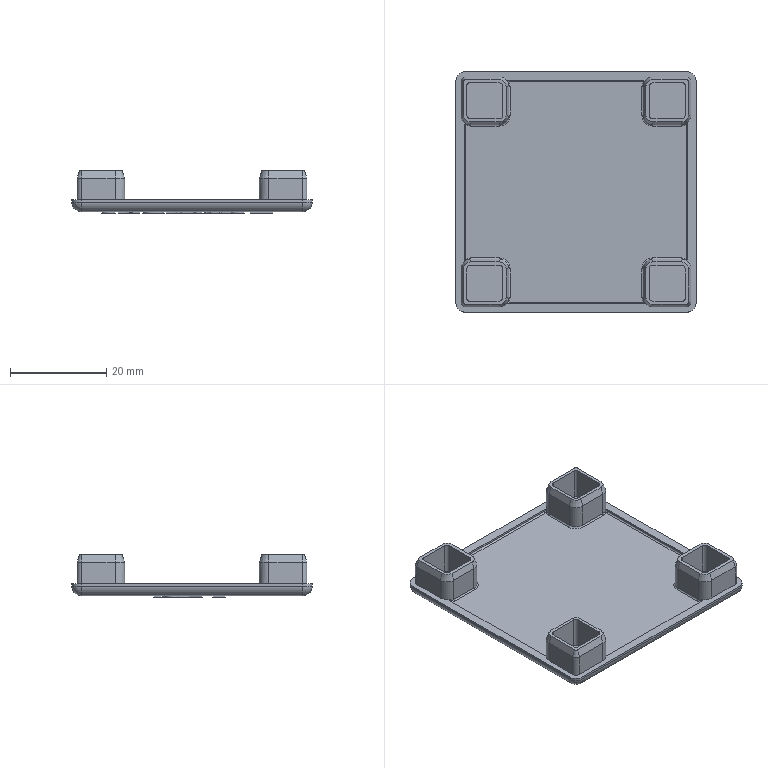Part | STEP file | 101000007578 | 1 solid | 350 faces | box 50 x 50 x 8.8 mm | volume 5573 mm3 | plane 201 | cylinder 76 | spline 27 | sphere 18 | cone 16 | torus 12 | commonest cylinder face diameters 0.6 x24 4 x20 1.6 x12 1 x4 2 x4 0.448 x2